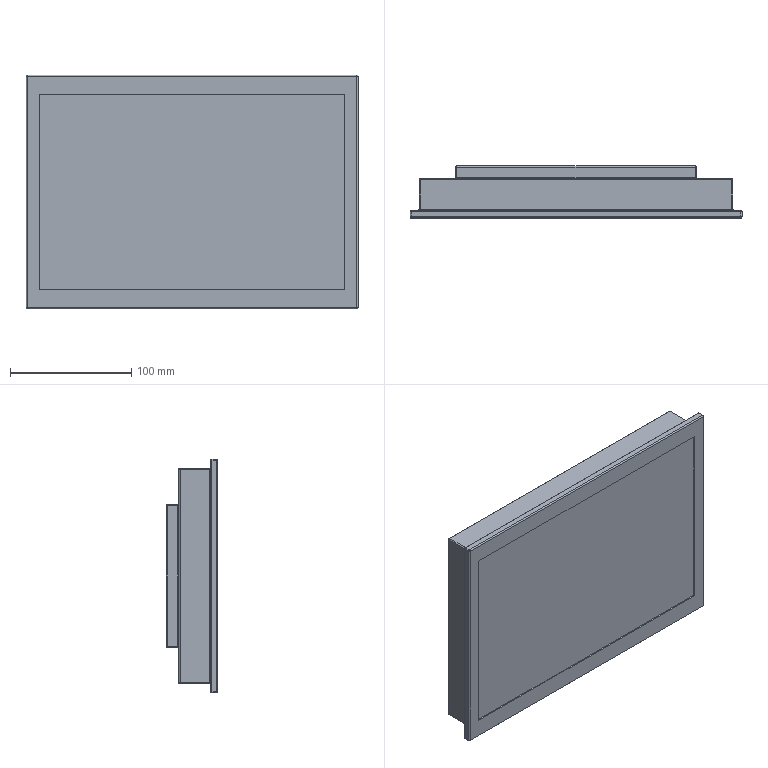Part | STEP file | Display screen | 1 solid | 78 faces | box 274 x 42.7 x 193 mm | volume 1730721 mm3 | cylinder 35 | plane 21 | sphere 15 | torus 7 | commonest cylinder face diameters 2 x35